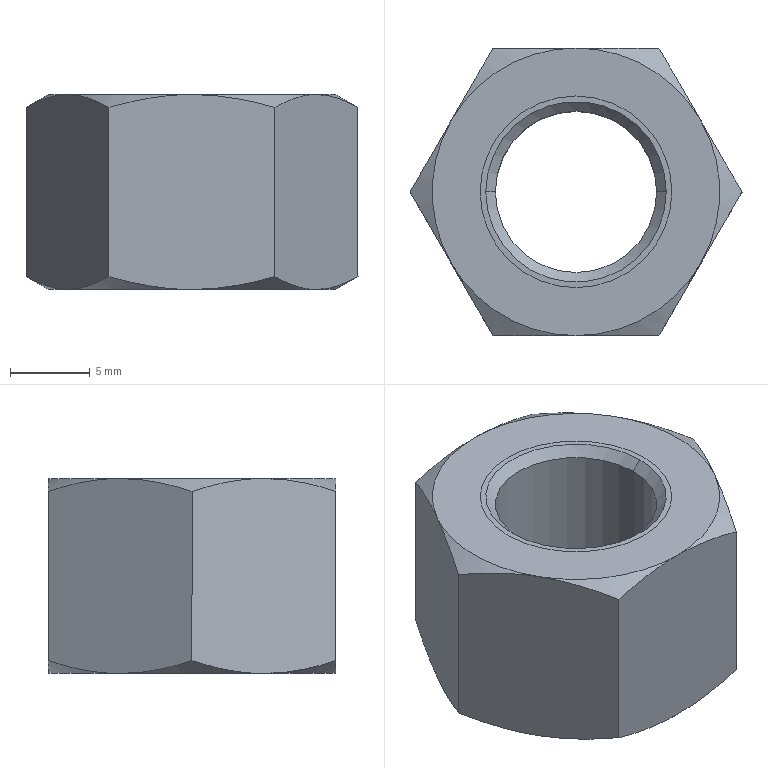Part | NX | features BREP 2 | 1 solid | 28 faces | box 20.785 x 18 x 12.2 mm | volume 3340 mm3 | cone 16 | plane 8 | cylinder 4 | commonest cylinder face diameters 10.106 x2 12 x2